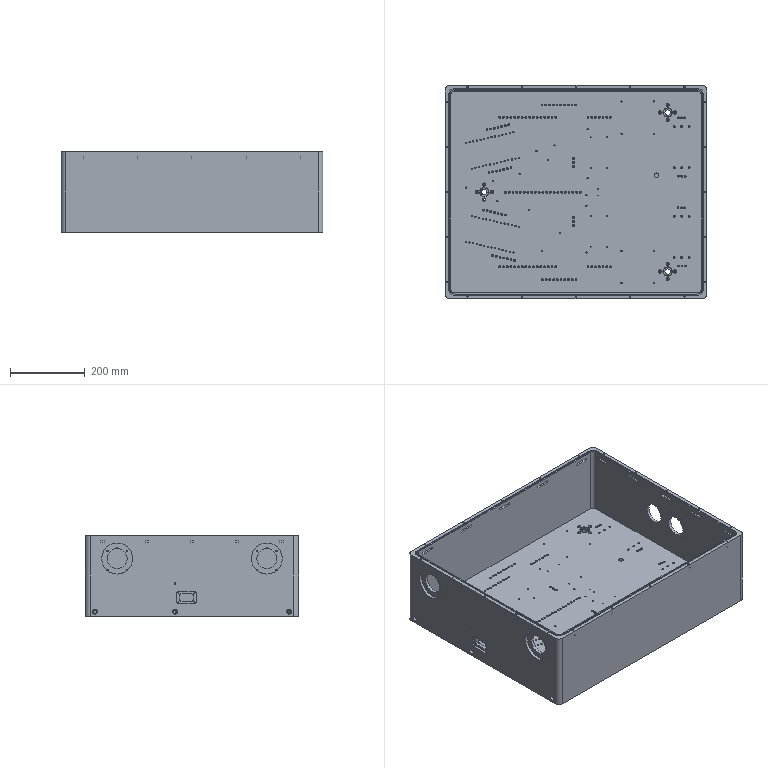Part | SolidWorks | features HoleWzd 21, Cut 16, ICE 8, MoveFace 6, Fillet 3, CutThin 2, Chamfer 1, Extrusion 1, Shell 1 | 3 solids | 1455 faces | box 700 x 570 x 215 mm | volume 18356109 mm3 | cylinder 732 | cone 584 | plane 139 | commonest cylinder face diameters 5 x290 3.3 x230 2.5 x28 40 x25 4.5 x24 8.5 x24